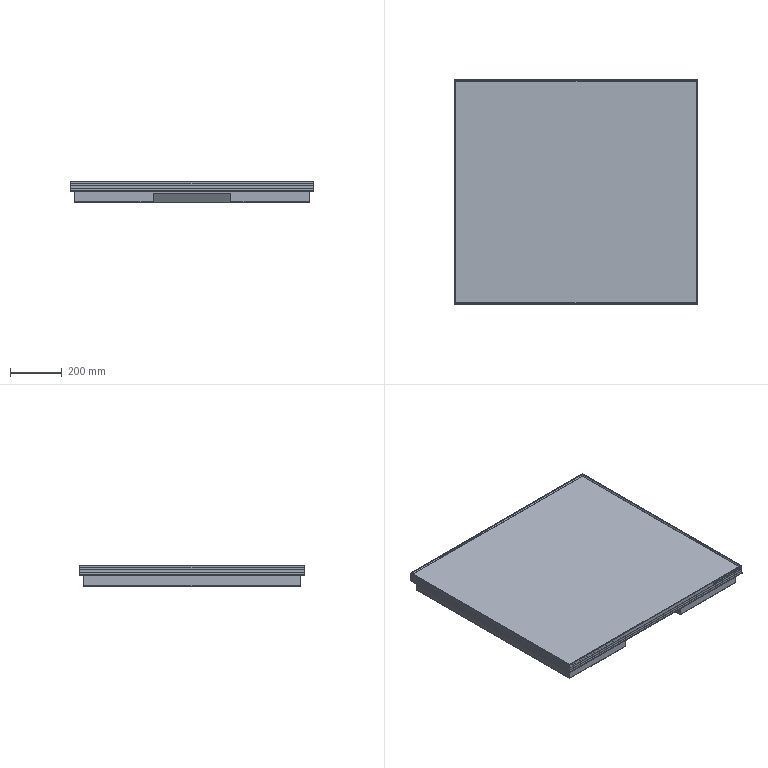Part | 8 solids | 408 faces | box 940 x 870 x 80 mm | volume 4538018 mm3 | plane 254 | cylinder 142 | spline 12 | commonest cylinder face diameters 7 x100 11 x16 1 x9 3 x9 5 x4 0.4 x2